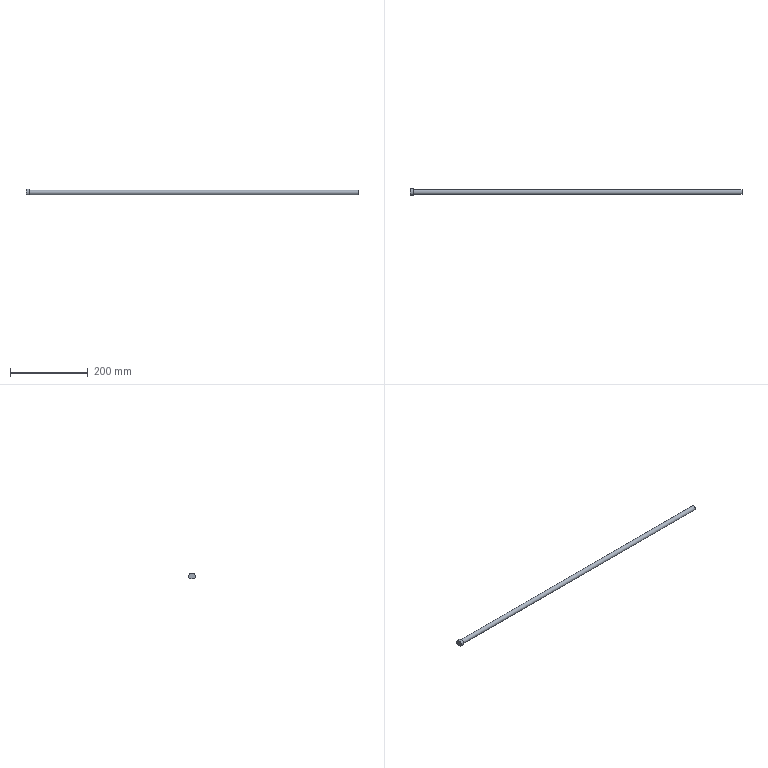Part | STEP file | solid 51 | 1 solid | 6 faces | box 855 x 17 x 15 mm | volume 97489 mm3 | plane 4 | cylinder 2 | commonest cylinder face diameters 12 x1 17 x1